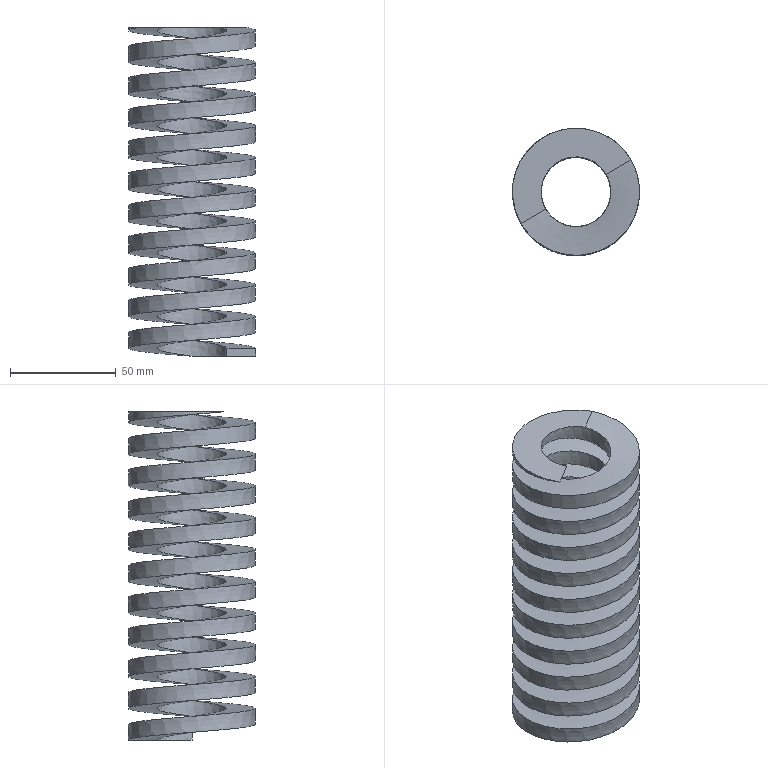Part | Creo | 1 solid | 7 faces | box 60 x 60 x 155 mm | volume 155284 mm3 | spline 4 | plane 3